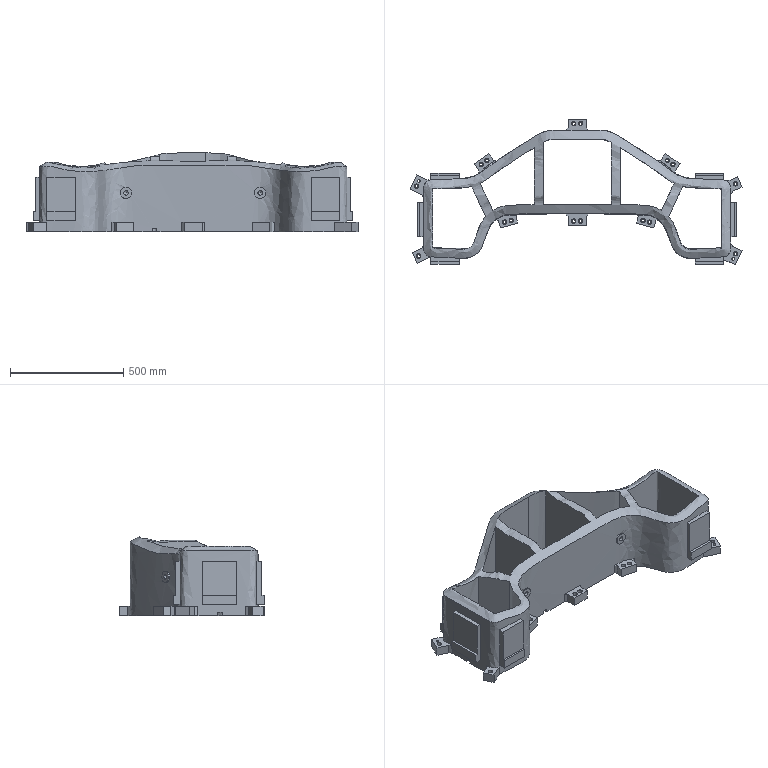Part | NX | features solid 2 | 1 solid | 197 faces | box 1464 x 643.32 x 349.11 mm | volume 85176838 mm3 | plane 138 | cylinder 43 | spline 12 | cone 4 | commonest cylinder face diameters 13.5 x16 19.5 x16 20 x5 50 x4 12 x2